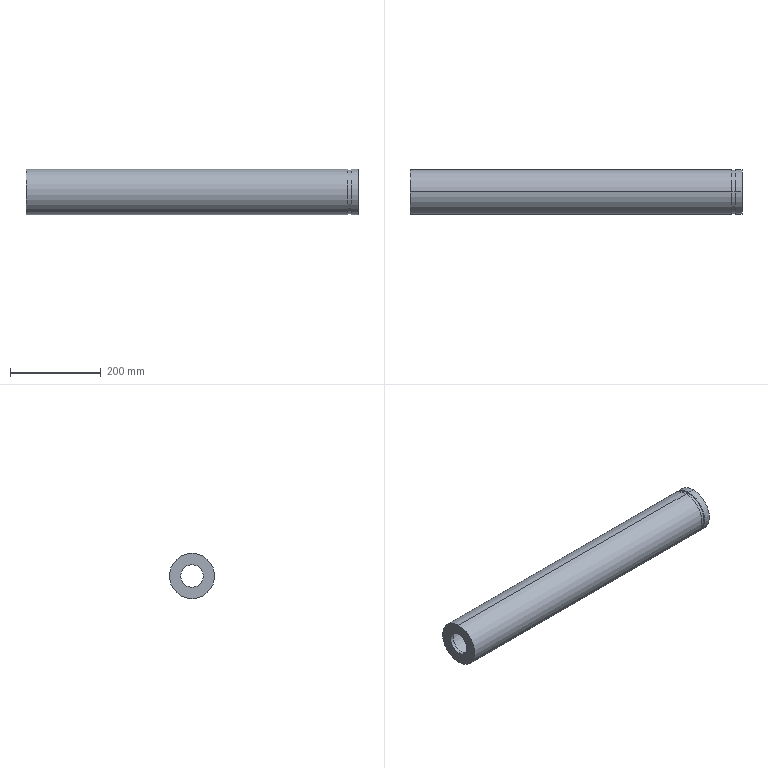Part | SolidWorks | features ICE 2, Revolution 1 | 1 solid | 15 faces | box 733.26 x 100 x 100 mm | volume 2092822 mm3 | cylinder 10 | plane 5 | commonest cylinder face diameters 100 x4 50 x2 80 x2 96 x2
STEP:
#1=CARTESIAN_POINT('',(-192.617,0.,-25.));
#2=VERTEX_POINT('',#1);
#3=CARTESIAN_POINT('',(-192.617,0.,25.));
#4=VERTEX_POINT('',#3);
#5=CARTESIAN_POINT('',(-192.617,0.,0.));
#6=DIRECTION('',(-1.,0.,0.));
#7=DIRECTION('',(0.,0.,1.));
#8=AXIS2_PLACEMENT_3D('',#5,#6,#7);
#9=CIRCLE('',#8,25.);
#10=EDGE_CURVE('',#2,#4,#9,.T.);
#11=ORIENTED_EDGE('',*,*,#10,.F.);
#12=CARTESIAN_POINT('',(-200.617,0.,-25.));
#13=VERTEX_POINT('',#12);
#14=CARTESIAN_POINT('',(-192.617,0.,-25.));
#15=DIRECTION('',(-1.,0.,0.));
#16=VECTOR('',#15,1000.);
#17=LINE('',#14,#16);
#18=EDGE_CURVE('',#2,#13,#17,.T.);
#19=ORIENTED_EDGE('',*,*,#18,.T.);
#20=CARTESIAN_POINT('',(-200.617,0.,25.));
#21=VERTEX_POINT('',#20);
#22=CARTESIAN_POINT('',(-200.617,0.,0.));
#23=DIRECTION('',(-1.,0.,0.));
#24=DIRECTION('',(0.,0.,1.));
#25=AXIS2_PLACEMENT_3D('',#22,#23,#24);
#26=CIRCLE('',#25,25.);
#27=EDGE_CURVE('',#13,#21,#26,.T.);
#28=ORIENTED_EDGE('',*,*,#27,.T.);
#29=CARTESIAN_POINT('',(-192.617,0.,25.));
#30=DIRECTION('',(-1.,0.,0.));
#31=VECTOR('',#30,1000.);
#32=LINE('',#29,#31);
#33=EDGE_CURVE('',#4,#21,#32,.T.);
#34=ORIENTED_EDGE('',*,*,#33,.F.);
#35=EDGE_LOOP('',(#11,#19,#28,#34));
#36=FACE_OUTER_BOUND('',#35,.T.);
#37=CARTESIAN_POINT('',(-192.617,0.,0.));
#38=DIRECTION('',(-1.,0.,0.));
#39=DIRECTION('',(0.,0.,1.));
#40=AXIS2_PLACEMENT_3D('',#37,#38,#39);
#41=CYLINDRICAL_SURFACE('',#40,25.);
#42=ADVANCED_FACE('',(#36),#41,.F.);
#43=CARTESIAN_POINT('',(509.643,0.,50.));
#44=VERTEX_POINT('',#43);
#45=CARTESIAN_POINT('',(509.643,0.,-50.));
#46=VERTEX_POINT('',#45);
#47=CARTESIAN_POINT('',(509.643,0.,0.));
#48=DIRECTION('',(-1.,0.,0.));
#49=DIRECTION('',(0.,0.,1.));
#50=AXIS2_PLACEMENT_3D('',#47,#48,#49);
#51=CIRCLE('',#50,50.);
#52=EDGE_CURVE('',#44,#46,#51,.T.);
#53=ORIENTED_EDGE('',*,*,#52,.T.);
#54=CARTESIAN_POINT('',(-200.617,0.,-50.));
#55=VERTEX_POINT('',#54);
#56=CARTESIAN_POINT('',(-27.214,0.,-50.));
#57=DIRECTION('',(-1.,0.,0.));
#58=VECTOR('',#57,1000.);
#59=LINE('',#56,#58);
#60=EDGE_CURVE('',#46,#55,#59,.T.);
#61=ORIENTED_EDGE('',*,*,#60,.T.);
#62=CARTESIAN_POINT('',(-200.617,0.,50.));
#63=VERTEX_POINT('',#62);
#64=CARTESIAN_POINT('',(-200.617,0.,0.));
#65=DIRECTION('',(-1.,0.,0.));
#66=DIRECTION('',(0.,0.,1.));
#67=AXIS2_PLACEMENT_3D('',#64,#65,#66);
#68=CIRCLE('',#67,50.);
#69=EDGE_CURVE('',#63,#55,#68,.T.);
#70=ORIENTED_EDGE('',*,*,#69,.F.);
#71=CARTESIAN_POINT('',(-27.214,0.,50.));
#72=DIRECTION('',(-1.,0.,0.));
#73=VECTOR('',#72,1000.);
#74=LINE('',#71,#73);
#75=EDGE_CURVE('',#44,#63,#74,.T.);
#76=ORIENTED_EDGE('',*,*,#75,.F.);
#77=EDGE_LOOP('',(#53,#61,#70,#76));
#78=FACE_OUTER_BOUND('',#77,.T.);
#79=CARTESIAN_POINT('',(-27.214,0.,0.));
#80=DIRECTION('',(-1.,0.,0.));
#81=DIRECTION('',(0.,0.,1.));
#82=AXIS2_PLACEMENT_3D('',#79,#80,#81);
#83=CYLINDRICAL_SURFACE('',#82,50.);
#84=ADVANCED_FACE('',(#78),#83,.T.);
#85=CARTESIAN_POINT('',(517.643,0.,48.));
#86=VERTEX_POINT('',#85);
#87=CARTESIAN_POINT('',(517.643,0.,-48.));
#88=VERTEX_POINT('',#87);
#89=CARTESIAN_POINT('',(517.643,0.,0.));
#90=DIRECTION('',(-1.,0.,0.));
#91=DIRECTION('',(0.,0.,1.));
#92=AXIS2_PLACEMENT_3D('',#89,#90,#91);
#93=CIRCLE('',#92,48.);
#94=EDGE_CURVE('',#86,#88,#93,.T.);
#95=ORIENTED_EDGE('',*,*,#94,.T.);
#96=CARTESIAN_POINT('',(509.643,0.,-48.));
#97=VERTEX_POINT('',#96);
#98=CARTESIAN_POINT('',(-27.214,0.,-48.));
#99=DIRECTION('',(-1.,0.,0.));
#100=VECTOR('',#99,1000.);
#101=LINE('',#98,#100);
#102=EDGE_CURVE('',#88,#97,#101,.T.);
#103=ORIENTED_EDGE('',*,*,#102,.T.);
#104=CARTESIAN_POINT('',(509.643,0.,48.));
#105=VERTEX_POINT('',#104);
#106=CARTESIAN_POINT('',(509.643,0.,0.));
#107=DIRECTION('',(-1.,0.,0.));
#108=DIRECTION('',(0.,0.,1.));
#109=AXIS2_PLACEMENT_3D('',#106,#107,#108);
#110=CIRCLE('',#109,48.);
#111=EDGE_CURVE('',#105,#97,#110,.T.);
#112=ORIENTED_EDGE('',*,*,#111,.F.);
#113=CARTESIAN_POINT('',(-27.214,0.,48.));
#114=DIRECTION('',(-1.,0.,0.));
#115=VECTOR('',#114,1000.);
#116=LINE('',#113,#115);
#117=EDGE_CURVE('',#86,#105,#116,.T.);
#118=ORIENTED_EDGE('',*,*,#117,.F.);
#119=EDGE_LOOP('',(#95,#103,#112,#118));
#120=FACE_OUTER_BOUND('',#119,.T.);
#121=CARTESIAN_POINT('',(-27.214,0.,0.));
#122=DIRECTION('',(-1.,0.,0.));
#123=DIRECTION('',(0.,0.,1.));
#124=AXIS2_PLACEMENT_3D('',#121,#122,#123);
#125=CYLINDRICAL_SURFACE('',#124,48.);
#126=ADVANCED_FACE('',(#120),#125,.T.);
#127=CARTESIAN_POINT('',(532.643,0.,50.));
#128=VERTEX_POINT('',#127);
#129=CARTESIAN_POINT('',(532.643,0.,-50.));
#130=VERTEX_POINT('',#129);
#131=CARTESIAN_POINT('',(532.643,0.,0.));
#132=DIRECTION('',(-1.,0.,0.));
#133=DIRECTION('',(0.,0.,1.));
#134=AXIS2_PLACEMENT_3D('',#131,#132,#133);
#135=CIRCLE('',#134,50.);
#136=EDGE_CURVE('',#128,#130,#135,.T.);
#137=ORIENTED_EDGE('',*,*,#136,.T.);
#138=CARTESIAN_POINT('',(517.643,0.,-50.));
#139=VERTEX_POINT('',#138);
#140=CARTESIAN_POINT('',(-27.214,0.,-50.));
#141=DIRECTION('',(-1.,0.,0.));
#142=VECTOR('',#141,1000.);
#143=LINE('',#140,#142);
#144=EDGE_CURVE('',#130,#139,#143,.T.);
#145=ORIENTED_EDGE('',*,*,#144,.T.);
#146=CARTESIAN_POINT('',(517.643,0.,50.));
#147=VERTEX_POINT('',#146);
#148=CARTESIAN_POINT('',(517.643,0.,0.));
#149=DIRECTION('',(-1.,0.,0.));
#150=DIRECTION('',(0.,0.,1.));
#151=AXIS2_PLACEMENT_3D('',#148,#149,#150);
#152=CIRCLE('',#151,50.);
#153=EDGE_CURVE('',#147,#139,#152,.T.);
#154=ORIENTED_EDGE('',*,*,#153,.F.);
#155=CARTESIAN_POINT('',(-27.214,0.,50.));
#156=DIRECTION('',(-1.,0.,0.));
#157=VECTOR('',#156,1000.);
#158=LINE('',#155,#157);
#159=EDGE_CURVE('',#128,#147,#158,.T.);
#160=ORIENTED_EDGE('',*,*,#159,.F.);
#161=EDGE_LOOP('',(#137,#145,#154,#160));
#162=FACE_OUTER_BOUND('',#161,.T.);
#163=CARTESIAN_POINT('',(-27.214,0.,0.));
#164=DIRECTION('',(-1.,0.,0.));
#165=DIRECTION('',(0.,0.,1.));
#166=AXIS2_PLACEMENT_3D('',#163,#164,#165);
#167=CYLINDRICAL_SURFACE('',#166,50.);
#168=ADVANCED_FACE('',(#162),#167,.T.);
#169=CARTESIAN_POINT('',(532.643,0.,-40.));
#170=VERTEX_POINT('',#169);
#171=CARTESIAN_POINT('',(532.643,0.,40.));
#172=VERTEX_POINT('',#171);
#173=CARTESIAN_POINT('',(532.643,0.,0.));
#174=DIRECTION('',(-1.,0.,0.));
#175=DIRECTION('',(0.,0.,1.));
#176=AXIS2_PLACEMENT_3D('',#173,#174,#175);
#177=CIRCLE('',#176,40.);
#178=EDGE_CURVE('',#170,#172,#177,.T.);
#179=ORIENTED_EDGE('',*,*,#178,.F.);
#180=CARTESIAN_POINT('',(-192.617,0.,-40.));
#181=VERTEX_POINT('',#180);
#182=CARTESIAN_POINT('',(-27.214,0.,-40.));
#183=DIRECTION('',(-1.,0.,0.));
#184=VECTOR('',#183,1000.);
#185=LINE('',#182,#184);
#186=EDGE_CURVE('',#170,#181,#185,.T.);
#187=ORIENTED_EDGE('',*,*,#186,.T.);
#188=CARTESIAN_POINT('',(-192.617,0.,40.));
#189=VERTEX_POINT('',#188);
#190=CARTESIAN_POINT('',(-192.617,0.,0.));
#191=DIRECTION('',(1.,0.,0.));
#192=DIRECTION('',(0.,0.,1.));
#193=AXIS2_PLACEMENT_3D('',#190,#191,#192);
#194=CIRCLE('',#193,40.);
#195=EDGE_CURVE('',#189,#181,#194,.T.);
#196=ORIENTED_EDGE('',*,*,#195,.F.);
#197=CARTESIAN_POINT('',(-27.214,0.,40.));
#198=DIRECTION('',(-1.,0.,0.));
#199=VECTOR('',#198,1000.);
#200=LINE('',#197,#199);
#201=EDGE_CURVE('',#172,#189,#200,.T.);
#202=ORIENTED_EDGE('',*,*,#201,.F.);
#203=EDGE_LOOP('',(#179,#187,#196,#202));
#204=FACE_OUTER_BOUND('',#203,.T.);
#205=CARTESIAN_POINT('',(-27.214,0.,0.));
#206=DIRECTION('',(-1.,0.,0.));
#207=DIRECTION('',(0.,0.,1.));
#208=AXIS2_PLACEMENT_3D('',#205,#206,#207);
#209=CYLINDRICAL_SURFACE('',#208,40.);
#210=ADVANCED_FACE('',(#204),#209,.F.);
#211=ORIENTED_EDGE('',*,*,#186,.F.);
#212=CARTESIAN_POINT('',(532.643,0.,0.));
#213=DIRECTION('',(-1.,0.,0.));
#214=DIRECTION('',(0.,0.,1.));
#215=AXIS2_PLACEMENT_3D('',#212,#213,#214);
#216=CIRCLE('',#215,40.);
#217=EDGE_CURVE('',#172,#170,#216,.T.);
#218=ORIENTED_EDGE('',*,*,#217,.F.);
#219=ORIENTED_EDGE('',*,*,#201,.T.);
#220=CARTESIAN_POINT('',(-192.617,0.,0.));
#221=DIRECTION('',(1.,0.,0.));
#222=DIRECTION('',(0.,0.,1.));
#223=AXIS2_PLACEMENT_3D('',#220,#221,#222);
#224=CIRCLE('',#223,40.);
#225=EDGE_CURVE('',#181,#189,#224,.T.);
#226=ORIENTED_EDGE('',*,*,#225,.F.);
#227=EDGE_LOOP('',(#211,#218,#219,#226));
#228=FACE_OUTER_BOUND('',#227,.T.);
#229=CARTESIAN_POINT('',(-27.214,0.,0.));
#230=DIRECTION('',(-1.,0.,0.));
#231=DIRECTION('',(0.,0.,1.));
#232=AXIS2_PLACEMENT_3D('',#229,#230,#231);
#233=CYLINDRICAL_SURFACE('',#232,40.);
#234=ADVANCED_FACE('',(#228),#233,.F.);
#235=ORIENTED_EDGE('',*,*,#136,.F.);
#236=CARTESIAN_POINT('',(532.643,0.,0.));
#237=DIRECTION('',(-1.,0.,0.));
#238=DIRECTION('',(0.,0.,1.));
#239=AXIS2_PLACEMENT_3D('',#236,#237,#238);
#240=CIRCLE('',#239,50.);
#241=EDGE_CURVE('',#130,#128,#240,.T.);
#242=ORIENTED_EDGE('',*,*,#241,.F.);
#243=EDGE_LOOP('',(#235,#242));
#244=FACE_OUTER_BOUND('',#243,.T.);
#245=ORIENTED_EDGE('',*,*,#217,.T.);
#246=ORIENTED_EDGE('',*,*,#178,.T.);
#247=EDGE_LOOP('',(#245,#246));
#248=FACE_BOUND('',#247,.T.);
#249=CARTESIAN_POINT('',(532.643,40.,0.));
#250=DIRECTION('',(-1.,0.,0.));
#251=DIRECTION('',(0.,0.,1.));
#252=AXIS2_PLACEMENT_3D('',#249,#250,#251);
#253=PLANE('',#252);
#254=ADVANCED_FACE('',(#244,#248),#253,.F.);
#255=ORIENTED_EDGE('',*,*,#144,.F.);
#256=ORIENTED_EDGE('',*,*,#241,.T.);
#257=ORIENTED_EDGE('',*,*,#159,.T.);
#258=CARTESIAN_POINT('',(517.643,0.,0.));
#259=DIRECTION('',(-1.,0.,0.));
#260=DIRECTION('',(0.,0.,1.));
#261=AXIS2_PLACEMENT_3D('',#258,#259,#260);
#262=CIRCLE('',#261,50.);
#263=EDGE_CURVE('',#139,#147,#262,.T.);
#264=ORIENTED_EDGE('',*,*,#263,.F.);
#265=EDGE_LOOP('',(#255,#256,#257,#264));
#266=FACE_OUTER_BOUND('',#265,.T.);
#267=CARTESIAN_POINT('',(-27.214,0.,0.));
#268=DIRECTION('',(-1.,0.,0.));
#269=DIRECTION('',(0.,0.,1.));
#270=AXIS2_PLACEMENT_3D('',#267,#268,#269);
#271=CYLINDRICAL_SURFACE('',#270,50.);
#272=ADVANCED_FACE('',(#266),#271,.T.);
#273=ORIENTED_EDGE('',*,*,#94,.F.);
#274=CARTESIAN_POINT('',(517.643,0.,0.));
#275=DIRECTION('',(-1.,0.,0.));
#276=DIRECTION('',(0.,0.,1.));
#277=AXIS2_PLACEMENT_3D('',#274,#275,#276);
#278=CIRCLE('',#277,48.);
#279=EDGE_CURVE('',#88,#86,#278,.T.);
#280=ORIENTED_EDGE('',*,*,#279,.F.);
#281=EDGE_LOOP('',(#273,#280));
#282=FACE_BOUND('',#281,.T.);
#283=ORIENTED_EDGE('',*,*,#153,.T.);
#284=ORIENTED_EDGE('',*,*,#263,.T.);
#285=EDGE_LOOP('',(#283,#284));
#286=FACE_OUTER_BOUND('',#285,.T.);
#287=CARTESIAN_POINT('',(517.643,50.,0.));
#288=DIRECTION('',(1.,0.,0.));
#289=DIRECTION('',(0.,0.,-1.));
#290=AXIS2_PLACEMENT_3D('',#287,#288,#289);
#291=PLANE('',#290);
#292=ADVANCED_FACE('',(#282,#286),#291,.F.);
#293=ORIENTED_EDGE('',*,*,#102,.F.);
#294=ORIENTED_EDGE('',*,*,#279,.T.);
#295=ORIENTED_EDGE('',*,*,#117,.T.);
#296=CARTESIAN_POINT('',(509.643,0.,0.));
#297=DIRECTION('',(-1.,0.,0.));
#298=DIRECTION('',(0.,0.,1.));
#299=AXIS2_PLACEMENT_3D('',#296,#297,#298);
#300=CIRCLE('',#299,48.);
#301=EDGE_CURVE('',#97,#105,#300,.T.);
#302=ORIENTED_EDGE('',*,*,#301,.F.);
#303=EDGE_LOOP('',(#293,#294,#295,#302));
#304=FACE_OUTER_BOUND('',#303,.T.);
#305=CARTESIAN_POINT('',(-27.214,0.,0.));
#306=DIRECTION('',(-1.,0.,0.));
#307=DIRECTION('',(0.,0.,1.));
#308=AXIS2_PLACEMENT_3D('',#305,#306,#307);
#309=CYLINDRICAL_SURFACE('',#308,48.);
#310=ADVANCED_FACE('',(#304),#309,.T.);
#311=ORIENTED_EDGE('',*,*,#52,.F.);
#312=CARTESIAN_POINT('',(509.643,0.,0.));
#313=DIRECTION('',(-1.,0.,0.));
#314=DIRECTION('',(0.,0.,1.));
#315=AXIS2_PLACEMENT_3D('',#312,#313,#314);
#316=CIRCLE('',#315,50.);
#317=EDGE_CURVE('',#46,#44,#316,.T.);
#318=ORIENTED_EDGE('',*,*,#317,.F.);
#319=EDGE_LOOP('',(#311,#318));
#320=FACE_OUTER_BOUND('',#319,.T.);
#321=ORIENTED_EDGE('',*,*,#111,.T.);
#322=ORIENTED_EDGE('',*,*,#301,.T.);
#323=EDGE_LOOP('',(#321,#322));
#324=FACE_BOUND('',#323,.T.);
#325=CARTESIAN_POINT('',(509.643,48.,0.));
#326=DIRECTION('',(-1.,0.,0.));
#327=DIRECTION('',(0.,0.,1.));
#328=AXIS2_PLACEMENT_3D('',#325,#326,#327);
#329=PLANE('',#328);
#330=ADVANCED_FACE('',(#320,#324),#329,.F.);
#331=ORIENTED_EDGE('',*,*,#69,.T.);
#332=CARTESIAN_POINT('',(-200.617,0.,0.));
#333=DIRECTION('',(-1.,0.,0.));
#334=DIRECTION('',(0.,0.,1.));
#335=AXIS2_PLACEMENT_3D('',#332,#333,#334);
#336=CIRCLE('',#335,50.);
#337=EDGE_CURVE('',#55,#63,#336,.T.);
#338=ORIENTED_EDGE('',*,*,#337,.T.);
#339=EDGE_LOOP('',(#331,#338));
#340=FACE_OUTER_BOUND('',#339,.T.);
#341=CARTESIAN_POINT('',(-200.617,0.,0.));
#342=DIRECTION('',(-1.,0.,0.));
#343=DIRECTION('',(0.,0.,1.));
#344=AXIS2_PLACEMENT_3D('',#341,#342,#343);
#345=CIRCLE('',#344,25.);
#346=EDGE_CURVE('',#21,#13,#345,.T.);
#347=ORIENTED_EDGE('',*,*,#346,.F.);
#348=ORIENTED_EDGE('',*,*,#27,.F.);
#349=EDGE_LOOP('',(#347,#348));
#350=FACE_BOUND('',#349,.T.);
#351=CARTESIAN_POINT('',(-200.617,0.,0.));
#352=DIRECTION('',(-1.,0.,0.));
#353=DIRECTION('',(0.,0.,1.));
#354=AXIS2_PLACEMENT_3D('',#351,#352,#353);
#355=PLANE('',#354);
#356=ADVANCED_FACE('',(#340,#350),#355,.T.);
#357=ORIENTED_EDGE('',*,*,#60,.F.);
#358=ORIENTED_EDGE('',*,*,#317,.T.);
#359=ORIENTED_EDGE('',*,*,#75,.T.);
#360=ORIENTED_EDGE('',*,*,#337,.F.);
#361=EDGE_LOOP('',(#357,#358,#359,#360));
#362=FACE_OUTER_BOUND('',#361,.T.);
#363=CARTESIAN_POINT('',(-27.214,0.,0.));
#364=DIRECTION('',(-1.,0.,0.));
#365=DIRECTION('',(0.,0.,1.));
#366=AXIS2_PLACEMENT_3D('',#363,#364,#365);
#367=CYLINDRICAL_SURFACE('',#366,50.);
#368=ADVANCED_FACE('',(#362),#367,.T.);
#369=CARTESIAN_POINT('',(-192.617,0.,0.));
#370=DIRECTION('',(-1.,0.,0.));
#371=DIRECTION('',(0.,0.,1.));
#372=AXIS2_PLACEMENT_3D('',#369,#370,#371);
#373=CIRCLE('',#372,25.);
#374=EDGE_CURVE('',#4,#2,#373,.T.);
#375=ORIENTED_EDGE('',*,*,#374,.T.);
#376=ORIENTED_EDGE('',*,*,#10,.T.);
#377=EDGE_LOOP('',(#375,#376));
#378=FACE_BOUND('',#377,.T.);
#379=ORIENTED_EDGE('',*,*,#195,.T.);
#380=ORIENTED_EDGE('',*,*,#225,.T.);
#381=EDGE_LOOP('',(#379,#380));
#382=FACE_OUTER_BOUND('',#381,.T.);
#383=CARTESIAN_POINT('',(-192.617,0.,0.));
#384=DIRECTION('',(-1.,0.,0.));
#385=DIRECTION('',(0.,0.,1.));
#386=AXIS2_PLACEMENT_3D('',#383,#384,#385);
#387=PLANE('',#386);
#388=ADVANCED_FACE('',(#378,#382),#387,.F.);
#389=ORIENTED_EDGE('',*,*,#18,.F.);
#390=ORIENTED_EDGE('',*,*,#374,.F.);
#391=ORIENTED_EDGE('',*,*,#33,.T.);
#392=ORIENTED_EDGE('',*,*,#346,.T.);
#393=EDGE_LOOP('',(#389,#390,#391,#392));
#394=FACE_OUTER_BOUND('',#393,.T.);
#395=CARTESIAN_POINT('',(-192.617,0.,0.));
#396=DIRECTION('',(-1.,0.,0.));
#397=DIRECTION('',(0.,0.,1.));
#398=AXIS2_PLACEMENT_3D('',#395,#396,#397);
#399=CYLINDRICAL_SURFACE('',#398,25.);
#400=ADVANCED_FACE('',(#394),#399,.F.);
#401=CLOSED_SHELL('',(#42,#84,#126,#168,#210,#234,#254,#272,#292,#310,#330,#356,#368,#388,#400));
#402=MANIFOLD_SOLID_BREP('',#401);
#403=CARTESIAN_POINT('',(0.,0.,0.));
#404=DIRECTION('',(0.,0.,1.));
#405=DIRECTION('',(1.,0.,0.));
#406=AXIS2_PLACEMENT_3D('',#403,#404,#405);
#407=(LENGTH_UNIT()NAMED_UNIT(*)SI_UNIT(.MILLI.,.METRE.));
#408=UNCERTAINTY_MEASURE_WITH_UNIT(LENGTH_MEASURE(0.00001),#407,'','');
#409=(NAMED_UNIT(*)PLANE_ANGLE_UNIT()SI_UNIT($,.RADIAN.));
#410=(NAMED_UNIT(*)SI_UNIT($,.STERADIAN.)SOLID_ANGLE_UNIT());
#411=(GEOMETRIC_REPRESENTATION_CONTEXT(3)GLOBAL_UNCERTAINTY_ASSIGNED_CONTEXT((#408))GLOBAL_UNIT_ASSIGNED_CONTEXT((#407,#409,#410))REPRESENTATION_CONTEXT('',''));
#412=ADVANCED_BREP_SHAPE_REPRESENTATION('',(#402,#406),#411);